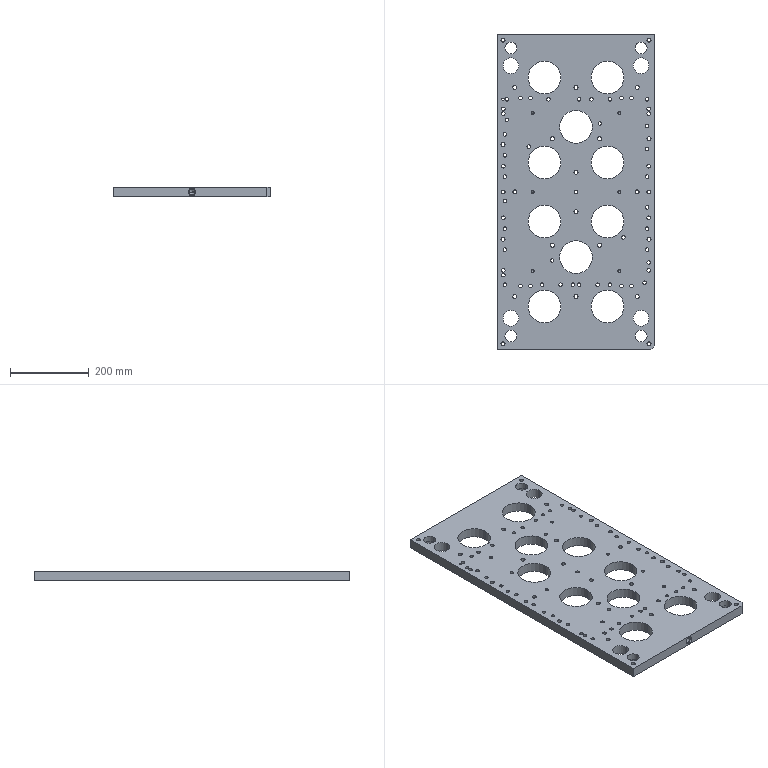Part | Creo | 1 solid | 440 faces | box 400 x 800 x 25 mm | volume 6250251 mm3 | cylinder 324 | plane 68 | cone 48 | commonest cylinder face diameters 9 x108 15 x101 10.2 x44 83 x20 6.8 x12 30.5 x8